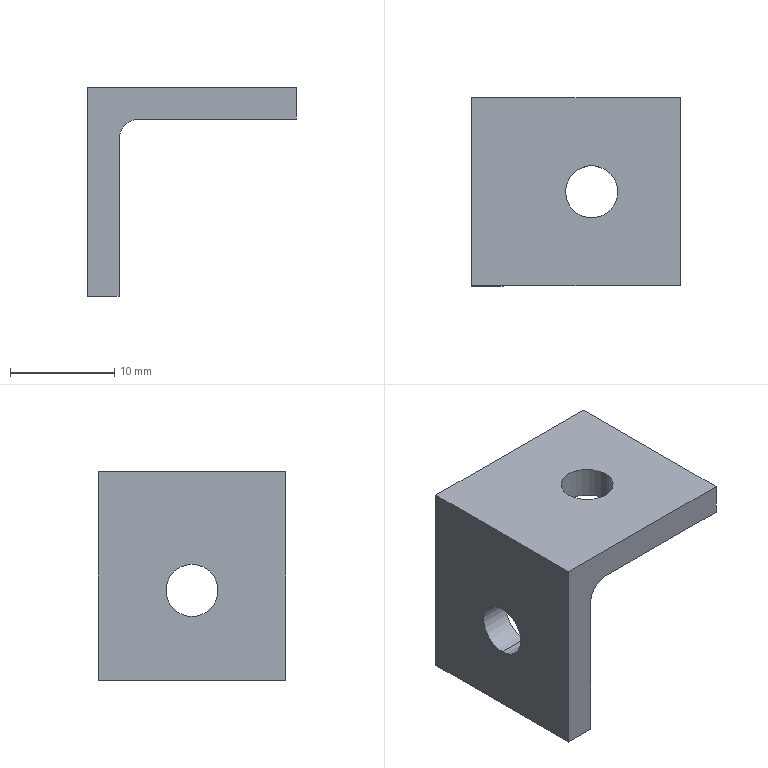Part | STEP file | 20 angle bracket flat | 1 solid | 13 faces | box 20 x 18 x 20 mm | volume 1896 mm3 | plane 8 | cylinder 5 | commonest cylinder face diameters 5 x4 4 x1
STEP:
#1=CARTESIAN_POINT('',(0.,0.,0.));
#2=DIRECTION('',(0.,0.,1.));
#3=DIRECTION('',(1.,0.,0.));
#4=AXIS2_PLACEMENT_3D('',#1,#2,#3);
#5=CARTESIAN_POINT('',(0.,9.,-13.886));
#6=VERTEX_POINT('',#5);
#7=CARTESIAN_POINT('',(3.,9.,-13.886));
#8=VERTEX_POINT('',#7);
#9=CARTESIAN_POINT('',(-7.,9.,-13.886));
#10=DIRECTION('',(1.,0.,0.));
#11=VECTOR('',#10,1.);
#12=LINE('',#9,#11);
#13=CARTESIAN_POINT('',(-7.,9.,-11.386));
#14=DIRECTION('',(1.,0.,0.));
#15=DIRECTION('',(0.,0.,-1.));
#16=AXIS2_PLACEMENT_3D('',#13,#14,#15);
#17=CYLINDRICAL_SURFACE('',#16,2.5);
#18=CARTESIAN_POINT('',(6.283,0.));
#19=DIRECTION('',(0.,1.));
#20=VECTOR('',#19,1.);
#21=LINE('',#18,#20);
#22=(GEOMETRIC_REPRESENTATION_CONTEXT(2)PARAMETRIC_REPRESENTATION_CONTEXT()REPRESENTATION_CONTEXT('',''));
#23=DEFINITIONAL_REPRESENTATION('',(#21),#22);
#24=PCURVE('',#17,#23);
#25=CARTESIAN_POINT('',(-7.,9.,-11.386));
#26=DIRECTION('',(1.,0.,0.));
#27=DIRECTION('',(0.,0.,-1.));
#28=AXIS2_PLACEMENT_3D('',#25,#26,#27);
#29=CYLINDRICAL_SURFACE('',#28,2.5);
#30=CARTESIAN_POINT('',(0.,0.));
#31=DIRECTION('',(0.,1.));
#32=VECTOR('',#31,1.);
#33=LINE('',#30,#32);
#34=(GEOMETRIC_REPRESENTATION_CONTEXT(2)PARAMETRIC_REPRESENTATION_CONTEXT()REPRESENTATION_CONTEXT('',''));
#35=DEFINITIONAL_REPRESENTATION('',(#33),#34);
#36=PCURVE('',#29,#35);
#37=SURFACE_CURVE('',#12,(#24,#36),.PCURVE_S1.);
#38=EDGE_CURVE('',#6,#8,#37,.T.);
#39=ORIENTED_EDGE('',*,*,#38,.T.);
#40=CARTESIAN_POINT('',(3.,9.,-8.886));
#41=VERTEX_POINT('',#40);
#42=CARTESIAN_POINT('',(3.,9.,-11.386));
#43=DIRECTION('',(1.,0.,0.));
#44=DIRECTION('',(0.,0.,-1.));
#45=AXIS2_PLACEMENT_3D('',#42,#43,#44);
#46=CIRCLE('',#45,2.5);
#47=CARTESIAN_POINT('',(0.,10.));
#48=DIRECTION('',(1.,0.));
#49=VECTOR('',#48,1.);
#50=LINE('',#47,#49);
#51=(GEOMETRIC_REPRESENTATION_CONTEXT(2)PARAMETRIC_REPRESENTATION_CONTEXT()REPRESENTATION_CONTEXT('',''));
#52=DEFINITIONAL_REPRESENTATION('',(#50),#51);
#53=PCURVE('',#17,#52);
#54=CARTESIAN_POINT('',(3.,18.,-20.));
#55=DIRECTION('',(1.,0.,0.));
#56=DIRECTION('',(0.,0.,-1.));
#57=AXIS2_PLACEMENT_3D('',#54,#55,#56);
#58=PLANE('',#57);
#59=CARTESIAN_POINT('',(-8.614,-9.));
#60=DIRECTION('',(1.,0.));
#61=AXIS2_PLACEMENT_2D('',#59,#60);
#62=CIRCLE('',#61,2.5);
#63=(GEOMETRIC_REPRESENTATION_CONTEXT(2)PARAMETRIC_REPRESENTATION_CONTEXT()REPRESENTATION_CONTEXT('',''));
#64=DEFINITIONAL_REPRESENTATION('',(#62),#63);
#65=PCURVE('',#58,#64);
#66=SURFACE_CURVE('',#46,(#53,#65),.PCURVE_S1.);
#67=EDGE_CURVE('',#41,#8,#66,.T.);
#68=ORIENTED_EDGE('',*,*,#67,.F.);
#69=CARTESIAN_POINT('',(0.,9.,-8.886));
#70=VERTEX_POINT('',#69);
#71=CARTESIAN_POINT('',(-7.,9.,-8.886));
#72=DIRECTION('',(1.,0.,0.));
#73=VECTOR('',#72,1.);
#74=LINE('',#71,#73);
#75=CARTESIAN_POINT('',(3.142,0.));
#76=DIRECTION('',(0.,1.));
#77=VECTOR('',#76,1.);
#78=LINE('',#75,#77);
#79=(GEOMETRIC_REPRESENTATION_CONTEXT(2)PARAMETRIC_REPRESENTATION_CONTEXT()REPRESENTATION_CONTEXT('',''));
#80=DEFINITIONAL_REPRESENTATION('',(#78),#79);
#81=PCURVE('',#17,#80);
#82=CARTESIAN_POINT('',(3.142,0.));
#83=DIRECTION('',(0.,1.));
#84=VECTOR('',#83,1.);
#85=LINE('',#82,#84);
#86=(GEOMETRIC_REPRESENTATION_CONTEXT(2)PARAMETRIC_REPRESENTATION_CONTEXT()REPRESENTATION_CONTEXT('',''));
#87=DEFINITIONAL_REPRESENTATION('',(#85),#86);
#88=PCURVE('',#29,#87);
#89=SURFACE_CURVE('',#74,(#81,#88),.PCURVE_S1.);
#90=EDGE_CURVE('',#70,#41,#89,.T.);
#91=ORIENTED_EDGE('',*,*,#90,.F.);
#92=CARTESIAN_POINT('',(0.,9.,-11.386));
#93=DIRECTION('',(1.,0.,0.));
#94=DIRECTION('',(0.,0.,-1.));
#95=AXIS2_PLACEMENT_3D('',#92,#93,#94);
#96=CIRCLE('',#95,2.5);
#97=CARTESIAN_POINT('',(0.,7.));
#98=DIRECTION('',(1.,0.));
#99=VECTOR('',#98,1.);
#100=LINE('',#97,#99);
#101=(GEOMETRIC_REPRESENTATION_CONTEXT(2)PARAMETRIC_REPRESENTATION_CONTEXT()REPRESENTATION_CONTEXT('',''));
#102=DEFINITIONAL_REPRESENTATION('',(#100),#101);
#103=PCURVE('',#17,#102);
#104=CARTESIAN_POINT('',(0.,18.,-20.));
#105=DIRECTION('',(1.,0.,0.));
#106=DIRECTION('',(0.,0.,-1.));
#107=AXIS2_PLACEMENT_3D('',#104,#105,#106);
#108=PLANE('',#107);
#109=CARTESIAN_POINT('',(-8.614,-9.));
#110=DIRECTION('',(1.,0.));
#111=AXIS2_PLACEMENT_2D('',#109,#110);
#112=CIRCLE('',#111,2.5);
#113=(GEOMETRIC_REPRESENTATION_CONTEXT(2)PARAMETRIC_REPRESENTATION_CONTEXT()REPRESENTATION_CONTEXT('',''));
#114=DEFINITIONAL_REPRESENTATION('',(#112),#113);
#115=PCURVE('',#108,#114);
#116=SURFACE_CURVE('',#96,(#103,#115),.PCURVE_S1.);
#117=EDGE_CURVE('',#70,#6,#116,.T.);
#118=ORIENTED_EDGE('',*,*,#117,.T.);
#119=EDGE_LOOP('',(#39,#68,#91,#118));
#120=FACE_BOUND('',#119,.F.);
#121=ADVANCED_FACE('',(#120),#17,.F.);
#122=CARTESIAN_POINT('',(9.,9.,0.));
#123=VERTEX_POINT('',#122);
#124=CARTESIAN_POINT('',(9.,9.,-3.));
#125=VERTEX_POINT('',#124);
#126=CARTESIAN_POINT('',(9.,9.,7.));
#127=DIRECTION('',(0.,0.,-1.));
#128=VECTOR('',#127,1.);
#129=LINE('',#126,#128);
#130=CARTESIAN_POINT('',(11.5,9.,7.));
#131=DIRECTION('',(0.,0.,-1.));
#132=DIRECTION('',(-1.,0.,0.));
#133=AXIS2_PLACEMENT_3D('',#130,#131,#132);
#134=CYLINDRICAL_SURFACE('',#133,2.5);
#135=CARTESIAN_POINT('',(6.283,0.));
#136=DIRECTION('',(0.,1.));
#137=VECTOR('',#136,1.);
#138=LINE('',#135,#137);
#139=(GEOMETRIC_REPRESENTATION_CONTEXT(2)PARAMETRIC_REPRESENTATION_CONTEXT()REPRESENTATION_CONTEXT('',''));
#140=DEFINITIONAL_REPRESENTATION('',(#138),#139);
#141=PCURVE('',#134,#140);
#142=CARTESIAN_POINT('',(11.5,9.,7.));
#143=DIRECTION('',(0.,0.,-1.));
#144=DIRECTION('',(-1.,0.,0.));
#145=AXIS2_PLACEMENT_3D('',#142,#143,#144);
#146=CYLINDRICAL_SURFACE('',#145,2.5);
#147=CARTESIAN_POINT('',(0.,0.));
#148=DIRECTION('',(0.,1.));
#149=VECTOR('',#148,1.);
#150=LINE('',#147,#149);
#151=(GEOMETRIC_REPRESENTATION_CONTEXT(2)PARAMETRIC_REPRESENTATION_CONTEXT()REPRESENTATION_CONTEXT('',''));
#152=DEFINITIONAL_REPRESENTATION('',(#150),#151);
#153=PCURVE('',#146,#152);
#154=SURFACE_CURVE('',#129,(#141,#153),.PCURVE_S1.);
#155=EDGE_CURVE('',#123,#125,#154,.T.);
#156=ORIENTED_EDGE('',*,*,#155,.T.);
#157=CARTESIAN_POINT('',(14.,9.,-3.));
#158=VERTEX_POINT('',#157);
#159=CARTESIAN_POINT('',(11.5,9.,-3.));
#160=DIRECTION('',(0.,0.,-1.));
#161=DIRECTION('',(-1.,0.,0.));
#162=AXIS2_PLACEMENT_3D('',#159,#160,#161);
#163=CIRCLE('',#162,2.5);
#164=CARTESIAN_POINT('',(0.,10.));
#165=DIRECTION('',(1.,0.));
#166=VECTOR('',#165,1.);
#167=LINE('',#164,#166);
#168=(GEOMETRIC_REPRESENTATION_CONTEXT(2)PARAMETRIC_REPRESENTATION_CONTEXT()REPRESENTATION_CONTEXT('',''));
#169=DEFINITIONAL_REPRESENTATION('',(#167),#168);
#170=PCURVE('',#134,#169);
#171=CARTESIAN_POINT('',(0.,18.,-3.));
#172=DIRECTION('',(0.,0.,-1.));
#173=DIRECTION('',(-1.,0.,0.));
#174=AXIS2_PLACEMENT_3D('',#171,#172,#173);
#175=PLANE('',#174);
#176=CARTESIAN_POINT('',(-11.5,-9.));
#177=DIRECTION('',(1.,0.));
#178=AXIS2_PLACEMENT_2D('',#176,#177);
#179=CIRCLE('',#178,2.5);
#180=(GEOMETRIC_REPRESENTATION_CONTEXT(2)PARAMETRIC_REPRESENTATION_CONTEXT()REPRESENTATION_CONTEXT('',''));
#181=DEFINITIONAL_REPRESENTATION('',(#179),#180);
#182=PCURVE('',#175,#181);
#183=SURFACE_CURVE('',#163,(#170,#182),.PCURVE_S1.);
#184=EDGE_CURVE('',#158,#125,#183,.T.);
#185=ORIENTED_EDGE('',*,*,#184,.F.);
#186=CARTESIAN_POINT('',(14.,9.,0.));
#187=VERTEX_POINT('',#186);
#188=CARTESIAN_POINT('',(14.,9.,7.));
#189=DIRECTION('',(0.,0.,-1.));
#190=VECTOR('',#189,1.);
#191=LINE('',#188,#190);
#192=CARTESIAN_POINT('',(3.142,0.));
#193=DIRECTION('',(0.,1.));
#194=VECTOR('',#193,1.);
#195=LINE('',#192,#194);
#196=(GEOMETRIC_REPRESENTATION_CONTEXT(2)PARAMETRIC_REPRESENTATION_CONTEXT()REPRESENTATION_CONTEXT('',''));
#197=DEFINITIONAL_REPRESENTATION('',(#195),#196);
#198=PCURVE('',#134,#197);
#199=CARTESIAN_POINT('',(3.142,0.));
#200=DIRECTION('',(0.,1.));
#201=VECTOR('',#200,1.);
#202=LINE('',#199,#201);
#203=(GEOMETRIC_REPRESENTATION_CONTEXT(2)PARAMETRIC_REPRESENTATION_CONTEXT()REPRESENTATION_CONTEXT('',''));
#204=DEFINITIONAL_REPRESENTATION('',(#202),#203);
#205=PCURVE('',#146,#204);
#206=SURFACE_CURVE('',#191,(#198,#205),.PCURVE_S1.);
#207=EDGE_CURVE('',#187,#158,#206,.T.);
#208=ORIENTED_EDGE('',*,*,#207,.F.);
#209=CARTESIAN_POINT('',(11.5,9.,0.));
#210=DIRECTION('',(0.,0.,-1.));
#211=DIRECTION('',(-1.,0.,0.));
#212=AXIS2_PLACEMENT_3D('',#209,#210,#211);
#213=CIRCLE('',#212,2.5);
#214=CARTESIAN_POINT('',(0.,7.));
#215=DIRECTION('',(1.,0.));
#216=VECTOR('',#215,1.);
#217=LINE('',#214,#216);
#218=(GEOMETRIC_REPRESENTATION_CONTEXT(2)PARAMETRIC_REPRESENTATION_CONTEXT()REPRESENTATION_CONTEXT('',''));
#219=DEFINITIONAL_REPRESENTATION('',(#217),#218);
#220=PCURVE('',#134,#219);
#221=CARTESIAN_POINT('',(0.,18.,0.));
#222=DIRECTION('',(0.,0.,-1.));
#223=DIRECTION('',(-1.,0.,0.));
#224=AXIS2_PLACEMENT_3D('',#221,#222,#223);
#225=PLANE('',#224);
#226=CARTESIAN_POINT('',(-11.5,-9.));
#227=DIRECTION('',(1.,0.));
#228=AXIS2_PLACEMENT_2D('',#226,#227);
#229=CIRCLE('',#228,2.5);
#230=(GEOMETRIC_REPRESENTATION_CONTEXT(2)PARAMETRIC_REPRESENTATION_CONTEXT()REPRESENTATION_CONTEXT('',''));
#231=DEFINITIONAL_REPRESENTATION('',(#229),#230);
#232=PCURVE('',#225,#231);
#233=SURFACE_CURVE('',#213,(#220,#232),.PCURVE_S1.);
#234=EDGE_CURVE('',#187,#123,#233,.T.);
#235=ORIENTED_EDGE('',*,*,#234,.T.);
#236=EDGE_LOOP('',(#156,#185,#208,#235));
#237=FACE_BOUND('',#236,.F.);
#238=ADVANCED_FACE('',(#237),#134,.F.);
#239=CARTESIAN_POINT('',(11.5,9.,0.));
#240=DIRECTION('',(0.,0.,-1.));
#241=DIRECTION('',(-1.,0.,0.));
#242=AXIS2_PLACEMENT_3D('',#239,#240,#241);
#243=CIRCLE('',#242,2.5);
#244=CARTESIAN_POINT('',(-11.5,-9.));
#245=DIRECTION('',(1.,0.));
#246=AXIS2_PLACEMENT_2D('',#244,#245);
#247=CIRCLE('',#246,2.5);
#248=(GEOMETRIC_REPRESENTATION_CONTEXT(2)PARAMETRIC_REPRESENTATION_CONTEXT()REPRESENTATION_CONTEXT('',''));
#249=DEFINITIONAL_REPRESENTATION('',(#247),#248);
#250=PCURVE('',#225,#249);
#251=CARTESIAN_POINT('',(0.,7.));
#252=DIRECTION('',(1.,0.));
#253=VECTOR('',#252,1.);
#254=LINE('',#251,#253);
#255=(GEOMETRIC_REPRESENTATION_CONTEXT(2)PARAMETRIC_REPRESENTATION_CONTEXT()REPRESENTATION_CONTEXT('',''));
#256=DEFINITIONAL_REPRESENTATION('',(#254),#255);
#257=PCURVE('',#146,#256);
#258=SURFACE_CURVE('',#243,(#250,#257),.PCURVE_S1.);
#259=EDGE_CURVE('',#123,#187,#258,.T.);
#260=ORIENTED_EDGE('',*,*,#259,.T.);
#261=ORIENTED_EDGE('',*,*,#234,.T.);
#262=EDGE_LOOP('',(#260,#261));
#263=FACE_BOUND('',#262,.T.);
#264=CARTESIAN_POINT('',(0.,0.,0.));
#265=VERTEX_POINT('',#264);
#266=CARTESIAN_POINT('',(20.,0.,0.));
#267=VERTEX_POINT('',#266);
#268=CARTESIAN_POINT('',(0.,0.,0.));
#269=DIRECTION('',(1.,0.,0.));
#270=VECTOR('',#269,1.);
#271=LINE('',#268,#270);
#272=CARTESIAN_POINT('',(0.,-18.));
#273=DIRECTION('',(-1.,0.));
#274=VECTOR('',#273,1.);
#275=LINE('',#272,#274);
#276=(GEOMETRIC_REPRESENTATION_CONTEXT(2)PARAMETRIC_REPRESENTATION_CONTEXT()REPRESENTATION_CONTEXT('',''));
#277=DEFINITIONAL_REPRESENTATION('',(#275),#276);
#278=PCURVE('',#225,#277);
#279=CARTESIAN_POINT('',(0.,0.,0.));
#280=DIRECTION('',(0.,-1.,0.));
#281=DIRECTION('',(-1.,0.,0.));
#282=AXIS2_PLACEMENT_3D('',#279,#280,#281);
#283=PLANE('',#282);
#284=CARTESIAN_POINT('',(0.,0.));
#285=DIRECTION('',(-1.,0.));
#286=VECTOR('',#285,1.);
#287=LINE('',#284,#286);
#288=(GEOMETRIC_REPRESENTATION_CONTEXT(2)PARAMETRIC_REPRESENTATION_CONTEXT()REPRESENTATION_CONTEXT('',''));
#289=DEFINITIONAL_REPRESENTATION('',(#287),#288);
#290=PCURVE('',#283,#289);
#291=SURFACE_CURVE('',#271,(#278,#290),.PCURVE_S1.);
#292=EDGE_CURVE('',#265,#267,#291,.T.);
#293=ORIENTED_EDGE('',*,*,#292,.T.);
#294=CARTESIAN_POINT('',(20.,18.,0.));
#295=VERTEX_POINT('',#294);
#296=CARTESIAN_POINT('',(20.,18.,0.));
#297=DIRECTION('',(0.,-1.,0.));
#298=VECTOR('',#297,1.);
#299=LINE('',#296,#298);
#300=CARTESIAN_POINT('',(-20.,0.));
#301=DIRECTION('',(0.,-1.));
#302=VECTOR('',#301,1.);
#303=LINE('',#300,#302);
#304=(GEOMETRIC_REPRESENTATION_CONTEXT(2)PARAMETRIC_REPRESENTATION_CONTEXT()REPRESENTATION_CONTEXT('',''));
#305=DEFINITIONAL_REPRESENTATION('',(#303),#304);
#306=PCURVE('',#225,#305);
#307=CARTESIAN_POINT('',(20.,18.,-3.));
#308=DIRECTION('',(1.,0.,0.));
#309=DIRECTION('',(0.,0.,-1.));
#310=AXIS2_PLACEMENT_3D('',#307,#308,#309);
#311=PLANE('',#310);
#312=CARTESIAN_POINT('',(-3.,0.));
#313=DIRECTION('',(0.,-1.));
#314=VECTOR('',#313,1.);
#315=LINE('',#312,#314);
#316=(GEOMETRIC_REPRESENTATION_CONTEXT(2)PARAMETRIC_REPRESENTATION_CONTEXT()REPRESENTATION_CONTEXT('',''));
#317=DEFINITIONAL_REPRESENTATION('',(#315),#316);
#318=PCURVE('',#311,#317);
#319=SURFACE_CURVE('',#299,(#306,#318),.PCURVE_S1.);
#320=EDGE_CURVE('',#295,#267,#319,.T.);
#321=ORIENTED_EDGE('',*,*,#320,.F.);
#322=CARTESIAN_POINT('',(0.,18.,0.));
#323=VERTEX_POINT('',#322);
#324=CARTESIAN_POINT('',(0.,18.,0.));
#325=DIRECTION('',(1.,0.,0.));
#326=VECTOR('',#325,1.);
#327=LINE('',#324,#326);
#328=CARTESIAN_POINT('',(0.,0.));
#329=DIRECTION('',(-1.,0.));
#330=VECTOR('',#329,1.);
#331=LINE('',#328,#330);
#332=(GEOMETRIC_REPRESENTATION_CONTEXT(2)PARAMETRIC_REPRESENTATION_CONTEXT()REPRESENTATION_CONTEXT('',''));
#333=DEFINITIONAL_REPRESENTATION('',(#331),#332);
#334=PCURVE('',#225,#333);
#335=CARTESIAN_POINT('',(0.,18.,0.));
#336=DIRECTION('',(0.,-1.,0.));
#337=DIRECTION('',(-1.,0.,0.));
#338=AXIS2_PLACEMENT_3D('',#335,#336,#337);
#339=PLANE('',#338);
#340=CARTESIAN_POINT('',(0.,0.));
#341=DIRECTION('',(-1.,0.));
#342=VECTOR('',#341,1.);
#343=LINE('',#340,#342);
#344=(GEOMETRIC_REPRESENTATION_CONTEXT(2)PARAMETRIC_REPRESENTATION_CONTEXT()REPRESENTATION_CONTEXT('',''));
#345=DEFINITIONAL_REPRESENTATION('',(#343),#344);
#346=PCURVE('',#339,#345);
#347=SURFACE_CURVE('',#327,(#334,#346),.PCURVE_S1.);
#348=EDGE_CURVE('',#323,#295,#347,.T.);
#349=ORIENTED_EDGE('',*,*,#348,.F.);
#350=CARTESIAN_POINT('',(0.,18.,0.));
#351=DIRECTION('',(0.,-1.,0.));
#352=VECTOR('',#351,1.);
#353=LINE('',#350,#352);
#354=CARTESIAN_POINT('',(0.,0.));
#355=DIRECTION('',(0.,-1.));
#356=VECTOR('',#355,1.);
#357=LINE('',#354,#356);
#358=(GEOMETRIC_REPRESENTATION_CONTEXT(2)PARAMETRIC_REPRESENTATION_CONTEXT()REPRESENTATION_CONTEXT('',''));
#359=DEFINITIONAL_REPRESENTATION('',(#357),#358);
#360=PCURVE('',#225,#359);
#361=CARTESIAN_POINT('',(-20.,0.));
#362=DIRECTION('',(0.,-1.));
#363=VECTOR('',#362,1.);
#364=LINE('',#361,#363);
#365=(GEOMETRIC_REPRESENTATION_CONTEXT(2)PARAMETRIC_REPRESENTATION_CONTEXT()REPRESENTATION_CONTEXT('',''));
#366=DEFINITIONAL_REPRESENTATION('',(#364),#365);
#367=PCURVE('',#108,#366);
#368=SURFACE_CURVE('',#353,(#360,#367),.PCURVE_S1.);
#369=EDGE_CURVE('',#323,#265,#368,.T.);
#370=ORIENTED_EDGE('',*,*,#369,.T.);
#371=EDGE_LOOP('',(#293,#321,#349,#370));
#372=FACE_BOUND('',#371,.T.);
#373=ADVANCED_FACE('',(#263,#372),#225,.F.);
#374=CARTESIAN_POINT('',(20.,0.,-3.));
#375=VERTEX_POINT('',#374);
#376=CARTESIAN_POINT('',(20.,0.,-3.));
#377=DIRECTION('',(0.,0.,1.));
#378=VECTOR('',#377,1.);
#379=LINE('',#376,#378);
#380=CARTESIAN_POINT('',(0.,-18.));
#381=DIRECTION('',(-1.,0.));
#382=VECTOR('',#381,1.);
#383=LINE('',#380,#382);
#384=(GEOMETRIC_REPRESENTATION_CONTEXT(2)PARAMETRIC_REPRESENTATION_CONTEXT()REPRESENTATION_CONTEXT('',''));
#385=DEFINITIONAL_REPRESENTATION('',(#383),#384);
#386=PCURVE('',#311,#385);
#387=CARTESIAN_POINT('',(-20.,3.));
#388=DIRECTION('',(0.,-1.));
#389=VECTOR('',#388,1.);
#390=LINE('',#387,#389);
#391=(GEOMETRIC_REPRESENTATION_CONTEXT(2)PARAMETRIC_REPRESENTATION_CONTEXT()REPRESENTATION_CONTEXT('',''));
#392=DEFINITIONAL_REPRESENTATION('',(#390),#391);
#393=PCURVE('',#283,#392);
#394=SURFACE_CURVE('',#379,(#386,#393),.PCURVE_S1.);
#395=EDGE_CURVE('',#375,#267,#394,.T.);
#396=ORIENTED_EDGE('',*,*,#395,.F.);
#397=CARTESIAN_POINT('',(20.,18.,-3.));
#398=VERTEX_POINT('',#397);
#399=CARTESIAN_POINT('',(20.,18.,-3.));
#400=DIRECTION('',(0.,-1.,0.));
#401=VECTOR('',#400,1.);
#402=LINE('',#399,#401);
#403=CARTESIAN_POINT('',(0.,0.));
#404=DIRECTION('',(0.,-1.));
#405=VECTOR('',#404,1.);
#406=LINE('',#403,#405);
#407=(GEOMETRIC_REPRESENTATION_CONTEXT(2)PARAMETRIC_REPRESENTATION_CONTEXT()REPRESENTATION_CONTEXT('',''));
#408=DEFINITIONAL_REPRESENTATION('',(#406),#407);
#409=PCURVE('',#311,#408);
#410=CARTESIAN_POINT('',(-20.,0.));
#411=DIRECTION('',(0.,-1.));
#412=VECTOR('',#411,1.);
#413=LINE('',#410,#412);
#414=(GEOMETRIC_REPRESENTATION_CONTEXT(2)PARAMETRIC_REPRESENTATION_CONTEXT()REPRESENTATION_CONTEXT('',''));
#415=DEFINITIONAL_REPRESENTATION('',(#413),#414);
#416=PCURVE('',#175,#415);
#417=SURFACE_CURVE('',#402,(#409,#416),.PCURVE_S1.);
#418=EDGE_CURVE('',#398,#375,#417,.T.);
#419=ORIENTED_EDGE('',*,*,#418,.F.);
#420=CARTESIAN_POINT('',(20.,18.,-3.));
#421=DIRECTION('',(0.,0.,1.));
#422=VECTOR('',#421,1.);
#423=LINE('',#420,#422);
#424=CARTESIAN_POINT('',(0.,0.));
#425=DIRECTION('',(-1.,0.));
#426=VECTOR('',#425,1.);
#427=LINE('',#424,#426);
#428=(GEOMETRIC_REPRESENTATION_CONTEXT(2)PARAMETRIC_REPRESENTATION_CONTEXT()REPRESENTATION_CONTEXT('',''));
#429=DEFINITIONAL_REPRESENTATION('',(#427),#428);
#430=PCURVE('',#311,#429);
#431=CARTESIAN_POINT('',(-20.,3.));
#432=DIRECTION('',(0.,-1.));
#433=VECTOR('',#432,1.);
#434=LINE('',#431,#433);
#435=(GEOMETRIC_REPRESENTATION_CONTEXT(2)PARAMETRIC_REPRESENTATION_CONTEXT()REPRESENTATION_CONTEXT('',''));
#436=DEFINITIONAL_REPRESENTATION('',(#434),#435);
#437=PCURVE('',#339,#436);
#438=SURFACE_CURVE('',#423,(#430,#437),.PCURVE_S1.);
#439=EDGE_CURVE('',#398,#295,#438,.T.);
#440=ORIENTED_EDGE('',*,*,#439,.T.);
#441=ORIENTED_EDGE('',*,*,#320,.T.);
#442=EDGE_LOOP('',(#396,#419,#440,#441));
#443=FACE_BOUND('',#442,.T.);
#444=ADVANCED_FACE('',(#443),#311,.T.);
#445=CARTESIAN_POINT('',(11.5,9.,-3.));
#446=DIRECTION('',(0.,0.,-1.));
#447=DIRECTION('',(-1.,0.,0.));
#448=AXIS2_PLACEMENT_3D('',#445,#446,#447);
#449=CIRCLE('',#448,2.5);
#450=CARTESIAN_POINT('',(-11.5,-9.));
#451=DIRECTION('',(1.,0.));
#452=AXIS2_PLACEMENT_2D('',#450,#451);
#453=CIRCLE('',#452,2.5);
#454=(GEOMETRIC_REPRESENTATION_CONTEXT(2)PARAMETRIC_REPRESENTATION_CONTEXT()REPRESENTATION_CONTEXT('',''));
#455=DEFINITIONAL_REPRESENTATION('',(#453),#454);
#456=PCURVE('',#175,#455);
#457=CARTESIAN_POINT('',(0.,10.));
#458=DIRECTION('',(1.,0.));
#459=VECTOR('',#458,1.);
#460=LINE('',#457,#459);
#461=(GEOMETRIC_REPRESENTATION_CONTEXT(2)PARAMETRIC_REPRESENTATION_CONTEXT()REPRESENTATION_CONTEXT('',''));
#462=DEFINITIONAL_REPRESENTATION('',(#460),#461);
#463=PCURVE('',#146,#462);
#464=SURFACE_CURVE('',#449,(#456,#463),.PCURVE_S1.);
#465=EDGE_CURVE('',#125,#158,#464,.T.);
#466=ORIENTED_EDGE('',*,*,#465,.F.);
#467=ORIENTED_EDGE('',*,*,#184,.F.);
#468=EDGE_LOOP('',(#466,#467));
#469=FACE_BOUND('',#468,.T.);
#470=CARTESIAN_POINT('',(5.,0.,-3.));
#471=VERTEX_POINT('',#470);
#472=CARTESIAN_POINT('',(0.,0.,-3.));
#473=DIRECTION('',(1.,0.,0.));
#474=VECTOR('',#473,1.);
#475=LINE('',#472,#474);
#476=CARTESIAN_POINT('',(0.,-18.));
#477=DIRECTION('',(-1.,0.));
#478=VECTOR('',#477,1.);
#479=LINE('',#476,#478);
#480=(GEOMETRIC_REPRESENTATION_CONTEXT(2)PARAMETRIC_REPRESENTATION_CONTEXT()REPRESENTATION_CONTEXT('',''));
#481=DEFINITIONAL_REPRESENTATION('',(#479),#480);
#482=PCURVE('',#175,#481);
#483=CARTESIAN_POINT('',(0.,3.));
#484=DIRECTION('',(-1.,0.));
#485=VECTOR('',#484,1.);
#486=LINE('',#483,#485);
#487=(GEOMETRIC_REPRESENTATION_CONTEXT(2)PARAMETRIC_REPRESENTATION_CONTEXT()REPRESENTATION_CONTEXT('',''));
#488=DEFINITIONAL_REPRESENTATION('',(#486),#487);
#489=PCURVE('',#283,#488);
#490=SURFACE_CURVE('',#475,(#482,#489),.PCURVE_S1.);
#491=EDGE_CURVE('',#471,#375,#490,.T.);
#492=ORIENTED_EDGE('',*,*,#491,.F.);
#493=CARTESIAN_POINT('',(5.,18.,-3.));
#494=VERTEX_POINT('',#493);
#495=CARTESIAN_POINT('',(5.,18.,-3.));
#496=DIRECTION('',(0.,1.,0.));
#497=VECTOR('',#496,1.);
#498=LINE('',#495,#497);
#499=CARTESIAN_POINT('',(-5.,0.));
#500=DIRECTION('',(0.,1.));
#501=VECTOR('',#500,1.);
#502=LINE('',#499,#501);
#503=(GEOMETRIC_REPRESENTATION_CONTEXT(2)PARAMETRIC_REPRESENTATION_CONTEXT()REPRESENTATION_CONTEXT('',''));
#504=DEFINITIONAL_REPRESENTATION('',(#502),#503);
#505=PCURVE('',#175,#504);
#506=CARTESIAN_POINT('',(5.,18.,-5.));
#507=DIRECTION('',(0.,1.,0.));
#508=DIRECTION('',(0.,0.,1.));
#509=AXIS2_PLACEMENT_3D('',#506,#507,#508);
#510=CYLINDRICAL_SURFACE('',#509,2.);
#511=CARTESIAN_POINT('',(6.283,0.));
#512=DIRECTION('',(0.,1.));
#513=VECTOR('',#512,1.);
#514=LINE('',#511,#513);
#515=(GEOMETRIC_REPRESENTATION_CONTEXT(2)PARAMETRIC_REPRESENTATION_CONTEXT()REPRESENTATION_CONTEXT('',''));
#516=DEFINITIONAL_REPRESENTATION('',(#514),#515);
#517=PCURVE('',#510,#516);
#518=SURFACE_CURVE('',#498,(#505,#517),.PCURVE_S1.);
#519=EDGE_CURVE('',#471,#494,#518,.T.);
#520=ORIENTED_EDGE('',*,*,#519,.T.);
#521=CARTESIAN_POINT('',(0.,18.,-3.));
#522=DIRECTION('',(1.,0.,0.));
#523=VECTOR('',#522,1.);
#524=LINE('',#521,#523);
#525=CARTESIAN_POINT('',(0.,0.));
#526=DIRECTION('',(-1.,0.));
#527=VECTOR('',#526,1.);
#528=LINE('',#525,#527);
#529=(GEOMETRIC_REPRESENTATION_CONTEXT(2)PARAMETRIC_REPRESENTATION_CONTEXT()REPRESENTATION_CONTEXT('',''));
#530=DEFINITIONAL_REPRESENTATION('',(#528),#529);
#531=PCURVE('',#175,#530);
#532=CARTESIAN_POINT('',(0.,3.));
#533=DIRECTION('',(-1.,0.));
#534=VECTOR('',#533,1.);
#535=LINE('',#532,#534);
#536=(GEOMETRIC_REPRESENTATION_CONTEXT(2)PARAMETRIC_REPRESENTATION_CONTEXT()REPRESENTATION_CONTEXT('',''));
#537=DEFINITIONAL_REPRESENTATION('',(#535),#536);
#538=PCURVE('',#339,#537);
#539=SURFACE_CURVE('',#524,(#531,#538),.PCURVE_S1.);
#540=EDGE_CURVE('',#494,#398,#539,.T.);
#541=ORIENTED_EDGE('',*,*,#540,.T.);
#542=ORIENTED_EDGE('',*,*,#418,.T.);
#543=EDGE_LOOP('',(#492,#520,#541,#542));
#544=FACE_BOUND('',#543,.T.);
#545=ADVANCED_FACE('',(#469,#544),#175,.T.);
#546=CARTESIAN_POINT('',(3.,9.,-11.386));
#547=DIRECTION('',(1.,0.,0.));
#548=DIRECTION('',(0.,0.,-1.));
#549=AXIS2_PLACEMENT_3D('',#546,#547,#548);
#550=CIRCLE('',#549,2.5);
#551=CARTESIAN_POINT('',(-8.614,-9.));
#552=DIRECTION('',(1.,0.));
#553=AXIS2_PLACEMENT_2D('',#551,#552);
#554=CIRCLE('',#553,2.5);
#555=(GEOMETRIC_REPRESENTATION_CONTEXT(2)PARAMETRIC_REPRESENTATION_CONTEXT()REPRESENTATION_CONTEXT('',''));
#556=DEFINITIONAL_REPRESENTATION('',(#554),#555);
#557=PCURVE('',#58,#556);
#558=CARTESIAN_POINT('',(0.,10.));
#559=DIRECTION('',(1.,0.));
#560=VECTOR('',#559,1.);
#561=LINE('',#558,#560);
#562=(GEOMETRIC_REPRESENTATION_CONTEXT(2)PARAMETRIC_REPRESENTATION_CONTEXT()REPRESENTATION_CONTEXT('',''));
#563=DEFINITIONAL_REPRESENTATION('',(#561),#562);
#564=PCURVE('',#29,#563);
#565=SURFACE_CURVE('',#550,(#557,#564),.PCURVE_S1.);
#566=EDGE_CURVE('',#8,#41,#565,.T.);
#567=ORIENTED_EDGE('',*,*,#566,.F.);
#568=ORIENTED_EDGE('',*,*,#67,.F.);
#569=EDGE_LOOP('',(#567,#568));
#570=FACE_BOUND('',#569,.T.);
#571=CARTESIAN_POINT('',(3.,18.,-20.));
#572=VERTEX_POINT('',#571);
#573=CARTESIAN_POINT('',(3.,18.,-5.));
#574=VERTEX_POINT('',#573);
#575=CARTESIAN_POINT('',(3.,18.,-20.));
#576=DIRECTION('',(0.,0.,1.));
#577=VECTOR('',#576,1.);
#578=LINE('',#575,#577);
#579=CARTESIAN_POINT('',(0.,0.));
#580=DIRECTION('',(-1.,0.));
#581=VECTOR('',#580,1.);
#582=LINE('',#579,#581);
#583=(GEOMETRIC_REPRESENTATION_CONTEXT(2)PARAMETRIC_REPRESENTATION_CONTEXT()REPRESENTATION_CONTEXT('',''));
#584=DEFINITIONAL_REPRESENTATION('',(#582),#583);
#585=PCURVE('',#58,#584);
#586=CARTESIAN_POINT('',(-3.,20.));
#587=DIRECTION('',(0.,-1.));
#588=VECTOR('',#587,1.);
#589=LINE('',#586,#588);
#590=(GEOMETRIC_REPRESENTATION_CONTEXT(2)PARAMETRIC_REPRESENTATION_CONTEXT()REPRESENTATION_CONTEXT('',''));
#591=DEFINITIONAL_REPRESENTATION('',(#589),#590);
#592=PCURVE('',#339,#591);
#593=SURFACE_CURVE('',#578,(#585,#592),.PCURVE_S1.);
#594=EDGE_CURVE('',#572,#574,#593,.T.);
#595=ORIENTED_EDGE('',*,*,#594,.T.);
#596=CARTESIAN_POINT('',(3.,0.,-5.));
#597=VERTEX_POINT('',#596);
#598=CARTESIAN_POINT('',(3.,0.,-5.));
#599=DIRECTION('',(0.,-1.,0.));
#600=VECTOR('',#599,1.);
#601=LINE('',#598,#600);
#602=CARTESIAN_POINT('',(-15.,-18.));
#603=DIRECTION('',(0.,-1.));
#604=VECTOR('',#603,1.);
#605=LINE('',#602,#604);
#606=(GEOMETRIC_REPRESENTATION_CONTEXT(2)PARAMETRIC_REPRESENTATION_CONTEXT()REPRESENTATION_CONTEXT('',''));
#607=DEFINITIONAL_REPRESENTATION('',(#605),#606);
#608=PCURVE('',#58,#607);
#609=CARTESIAN_POINT('',(4.712,-18.));
#610=DIRECTION('',(0.,-1.));
#611=VECTOR('',#610,1.);
#612=LINE('',#609,#611);
#613=(GEOMETRIC_REPRESENTATION_CONTEXT(2)PARAMETRIC_REPRESENTATION_CONTEXT()REPRESENTATION_CONTEXT('',''));
#614=DEFINITIONAL_REPRESENTATION('',(#612),#613);
#615=PCURVE('',#510,#614);
#616=SURFACE_CURVE('',#601,(#608,#615),.PCURVE_S1.);
#617=EDGE_CURVE('',#574,#597,#616,.T.);
#618=ORIENTED_EDGE('',*,*,#617,.T.);
#619=CARTESIAN_POINT('',(3.,0.,-20.));
#620=VERTEX_POINT('',#619);
#621=CARTESIAN_POINT('',(3.,0.,-20.));
#622=DIRECTION('',(0.,0.,1.));
#623=VECTOR('',#622,1.);
#624=LINE('',#621,#623);
#625=CARTESIAN_POINT('',(0.,-18.));
#626=DIRECTION('',(-1.,0.));
#627=VECTOR('',#626,1.);
#628=LINE('',#625,#627);
#629=(GEOMETRIC_REPRESENTATION_CONTEXT(2)PARAMETRIC_REPRESENTATION_CONTEXT()REPRESENTATION_CONTEXT('',''));
#630=DEFINITIONAL_REPRESENTATION('',(#628),#629);
#631=PCURVE('',#58,#630);
#632=CARTESIAN_POINT('',(-3.,20.));
#633=DIRECTION('',(0.,-1.));
#634=VECTOR('',#633,1.);
#635=LINE('',#632,#634);
#636=(GEOMETRIC_REPRESENTATION_CONTEXT(2)PARAMETRIC_REPRESENTATION_CONTEXT()REPRESENTATION_CONTEXT('',''));
#637=DEFINITIONAL_REPRESENTATION('',(#635),#636);
#638=PCURVE('',#283,#637);
#639=SURFACE_CURVE('',#624,(#631,#638),.PCURVE_S1.);
#640=EDGE_CURVE('',#620,#597,#639,.T.);
#641=ORIENTED_EDGE('',*,*,#640,.F.);
#642=CARTESIAN_POINT('',(3.,18.,-20.));
#643=DIRECTION('',(0.,-1.,0.));
#644=VECTOR('',#643,1.);
#645=LINE('',#642,#644);
#646=CARTESIAN_POINT('',(0.,0.));
#647=DIRECTION('',(0.,-1.));
#648=VECTOR('',#647,1.);
#649=LINE('',#646,#648);
#650=(GEOMETRIC_REPRESENTATION_CONTEXT(2)PARAMETRIC_REPRESENTATION_CONTEXT()REPRESENTATION_CONTEXT('',''));
#651=DEFINITIONAL_REPRESENTATION('',(#649),#650);
#652=PCURVE('',#58,#651);
#653=CARTESIAN_POINT('',(0.,18.,-20.));
#654=DIRECTION('',(0.,0.,-1.));
#655=DIRECTION('',(-1.,0.,0.));
#656=AXIS2_PLACEMENT_3D('',#653,#654,#655);
#657=PLANE('',#656);
#658=CARTESIAN_POINT('',(-3.,0.));
#659=DIRECTION('',(0.,-1.));
#660=VECTOR('',#659,1.);
#661=LINE('',#658,#660);
#662=(GEOMETRIC_REPRESENTATION_CONTEXT(2)PARAMETRIC_REPRESENTATION_CONTEXT()REPRESENTATION_CONTEXT('',''));
#663=DEFINITIONAL_REPRESENTATION('',(#661),#662);
#664=PCURVE('',#657,#663);
#665=SURFACE_CURVE('',#645,(#652,#664),.PCURVE_S1.);
#666=EDGE_CURVE('',#572,#620,#665,.T.);
#667=ORIENTED_EDGE('',*,*,#666,.F.);
#668=EDGE_LOOP('',(#595,#618,#641,#667));
#669=FACE_BOUND('',#668,.T.);
#670=ADVANCED_FACE('',(#570,#669),#58,.T.);
#671=CARTESIAN_POINT('',(0.,0.,-20.));
#672=VERTEX_POINT('',#671);
#673=CARTESIAN_POINT('',(0.,0.,-20.));
#674=DIRECTION('',(1.,0.,0.));
#675=VECTOR('',#674,1.);
#676=LINE('',#673,#675);
#677=CARTESIAN_POINT('',(0.,-18.));
#678=DIRECTION('',(-1.,0.));
#679=VECTOR('',#678,1.);
#680=LINE('',#677,#679);
#681=(GEOMETRIC_REPRESENTATION_CONTEXT(2)PARAMETRIC_REPRESENTATION_CONTEXT()REPRESENTATION_CONTEXT('',''));
#682=DEFINITIONAL_REPRESENTATION('',(#680),#681);
#683=PCURVE('',#657,#682);
#684=CARTESIAN_POINT('',(0.,20.));
#685=DIRECTION('',(-1.,0.));
#686=VECTOR('',#685,1.);
#687=LINE('',#684,#686);
#688=(GEOMETRIC_REPRESENTATION_CONTEXT(2)PARAMETRIC_REPRESENTATION_CONTEXT()REPRESENTATION_CONTEXT('',''));
#689=DEFINITIONAL_REPRESENTATION('',(#687),#688);
#690=PCURVE('',#283,#689);
#691=SURFACE_CURVE('',#676,(#683,#690),.PCURVE_S1.);
#692=EDGE_CURVE('',#672,#620,#691,.T.);
#693=ORIENTED_EDGE('',*,*,#692,.F.);
#694=CARTESIAN_POINT('',(0.,18.,-20.));
#695=VERTEX_POINT('',#694);
#696=CARTESIAN_POINT('',(0.,18.,-20.));
#697=DIRECTION('',(0.,-1.,0.));
#698=VECTOR('',#697,1.);
#699=LINE('',#696,#698);
#700=CARTESIAN_POINT('',(0.,0.));
#701=DIRECTION('',(0.,-1.));
#702=VECTOR('',#701,1.);
#703=LINE('',#700,#702);
#704=(GEOMETRIC_REPRESENTATION_CONTEXT(2)PARAMETRIC_REPRESENTATION_CONTEXT()REPRESENTATION_CONTEXT('',''));
#705=DEFINITIONAL_REPRESENTATION('',(#703),#704);
#706=PCURVE('',#657,#705);
#707=CARTESIAN_POINT('',(0.,0.));
#708=DIRECTION('',(0.,-1.));
#709=VECTOR('',#708,1.);
#710=LINE('',#707,#709);
#711=(GEOMETRIC_REPRESENTATION_CONTEXT(2)PARAMETRIC_REPRESENTATION_CONTEXT()REPRESENTATION_CONTEXT('',''));
#712=DEFINITIONAL_REPRESENTATION('',(#710),#711);
#713=PCURVE('',#108,#712);
#714=SURFACE_CURVE('',#699,(#706,#713),.PCURVE_S1.);
#715=EDGE_CURVE('',#695,#672,#714,.T.);
#716=ORIENTED_EDGE('',*,*,#715,.F.);
#717=CARTESIAN_POINT('',(0.,18.,-20.));
#718=DIRECTION('',(1.,0.,0.));
#719=VECTOR('',#718,1.);
#720=LINE('',#717,#719);
#721=CARTESIAN_POINT('',(0.,0.));
#722=DIRECTION('',(-1.,0.));
#723=VECTOR('',#722,1.);
#724=LINE('',#721,#723);
#725=(GEOMETRIC_REPRESENTATION_CONTEXT(2)PARAMETRIC_REPRESENTATION_CONTEXT()REPRESENTATION_CONTEXT('',''));
#726=DEFINITIONAL_REPRESENTATION('',(#724),#725);
#727=PCURVE('',#657,#726);
#728=CARTESIAN_POINT('',(0.,20.));
#729=DIRECTION('',(-1.,0.));
#730=VECTOR('',#729,1.);
#731=LINE('',#728,#730);
#732=(GEOMETRIC_REPRESENTATION_CONTEXT(2)PARAMETRIC_REPRESENTATION_CONTEXT()REPRESENTATION_CONTEXT('',''));
#733=DEFINITIONAL_REPRESENTATION('',(#731),#732);
#734=PCURVE('',#339,#733);
#735=SURFACE_CURVE('',#720,(#727,#734),.PCURVE_S1.);
#736=EDGE_CURVE('',#695,#572,#735,.T.);
#737=ORIENTED_EDGE('',*,*,#736,.T.);
#738=ORIENTED_EDGE('',*,*,#666,.T.);
#739=EDGE_LOOP('',(#693,#716,#737,#738));
#740=FACE_BOUND('',#739,.T.);
#741=ADVANCED_FACE('',(#740),#657,.T.);
#742=CARTESIAN_POINT('',(0.,9.,-11.386));
#743=DIRECTION('',(1.,0.,0.));
#744=DIRECTION('',(0.,0.,-1.));
#745=AXIS2_PLACEMENT_3D('',#742,#743,#744);
#746=CIRCLE('',#745,2.5);
#747=CARTESIAN_POINT('',(-8.614,-9.));
#748=DIRECTION('',(1.,0.));
#749=AXIS2_PLACEMENT_2D('',#747,#748);
#750=CIRCLE('',#749,2.5);
#751=(GEOMETRIC_REPRESENTATION_CONTEXT(2)PARAMETRIC_REPRESENTATION_CONTEXT()REPRESENTATION_CONTEXT('',''));
#752=DEFINITIONAL_REPRESENTATION('',(#750),#751);
#753=PCURVE('',#108,#752);
#754=CARTESIAN_POINT('',(0.,7.));
#755=DIRECTION('',(1.,0.));
#756=VECTOR('',#755,1.);
#757=LINE('',#754,#756);
#758=(GEOMETRIC_REPRESENTATION_CONTEXT(2)PARAMETRIC_REPRESENTATION_CONTEXT()REPRESENTATION_CONTEXT('',''));
#759=DEFINITIONAL_REPRESENTATION('',(#757),#758);
#760=PCURVE('',#29,#759);
#761=SURFACE_CURVE('',#746,(#753,#760),.PCURVE_S1.);
#762=EDGE_CURVE('',#6,#70,#761,.T.);
#763=ORIENTED_EDGE('',*,*,#762,.T.);
#764=ORIENTED_EDGE('',*,*,#117,.T.);
#765=EDGE_LOOP('',(#763,#764));
#766=FACE_BOUND('',#765,.T.);
#767=CARTESIAN_POINT('',(0.,0.,-20.));
#768=DIRECTION('',(0.,0.,1.));
#769=VECTOR('',#768,1.);
#770=LINE('',#767,#769);
#771=CARTESIAN_POINT('',(0.,-18.));
#772=DIRECTION('',(-1.,0.));
#773=VECTOR('',#772,1.);
#774=LINE('',#771,#773);
#775=(GEOMETRIC_REPRESENTATION_CONTEXT(2)PARAMETRIC_REPRESENTATION_CONTEXT()REPRESENTATION_CONTEXT('',''));
#776=DEFINITIONAL_REPRESENTATION('',(#774),#775);
#777=PCURVE('',#108,#776);
#778=CARTESIAN_POINT('',(0.,20.));
#779=DIRECTION('',(0.,-1.));
#780=VECTOR('',#779,1.);
#781=LINE('',#778,#780);
#782=(GEOMETRIC_REPRESENTATION_CONTEXT(2)PARAMETRIC_REPRESENTATION_CONTEXT()REPRESENTATION_CONTEXT('',''));
#783=DEFINITIONAL_REPRESENTATION('',(#781),#782);
#784=PCURVE('',#283,#783);
#785=SURFACE_CURVE('',#770,(#777,#784),.PCURVE_S1.);
#786=EDGE_CURVE('',#672,#265,#785,.T.);
#787=ORIENTED_EDGE('',*,*,#786,.T.);
#788=ORIENTED_EDGE('',*,*,#369,.F.);
#789=CARTESIAN_POINT('',(0.,18.,-20.));
#790=DIRECTION('',(0.,0.,1.));
#791=VECTOR('',#790,1.);
#792=LINE('',#789,#791);
#793=CARTESIAN_POINT('',(0.,0.));
#794=DIRECTION('',(-1.,0.));
#795=VECTOR('',#794,1.);
#796=LINE('',#793,#795);
#797=(GEOMETRIC_REPRESENTATION_CONTEXT(2)PARAMETRIC_REPRESENTATION_CONTEXT()REPRESENTATION_CONTEXT('',''));
#798=DEFINITIONAL_REPRESENTATION('',(#796),#797);
#799=PCURVE('',#108,#798);
#800=CARTESIAN_POINT('',(0.,20.));
#801=DIRECTION('',(0.,-1.));
#802=VECTOR('',#801,1.);
#803=LINE('',#800,#802);
#804=(GEOMETRIC_REPRESENTATION_CONTEXT(2)PARAMETRIC_REPRESENTATION_CONTEXT()REPRESENTATION_CONTEXT('',''));
#805=DEFINITIONAL_REPRESENTATION('',(#803),#804);
#806=PCURVE('',#339,#805);
#807=SURFACE_CURVE('',#792,(#799,#806),.PCURVE_S1.);
#808=EDGE_CURVE('',#695,#323,#807,.T.);
#809=ORIENTED_EDGE('',*,*,#808,.F.);
#810=ORIENTED_EDGE('',*,*,#715,.T.);
#811=EDGE_LOOP('',(#787,#788,#809,#810));
#812=FACE_BOUND('',#811,.T.);
#813=ADVANCED_FACE('',(#766,#812),#108,.F.);
#814=ORIENTED_EDGE('',*,*,#348,.T.);
#815=ORIENTED_EDGE('',*,*,#439,.F.);
#816=ORIENTED_EDGE('',*,*,#540,.F.);
#817=CARTESIAN_POINT('',(5.,18.,-5.));
#818=DIRECTION('',(0.,-1.,0.));
#819=DIRECTION('',(0.,0.,-1.));
#820=AXIS2_PLACEMENT_3D('',#817,#818,#819);
#821=CIRCLE('',#820,2.);
#822=CARTESIAN_POINT('',(-5.,5.));
#823=DIRECTION('',(0.,1.));
#824=AXIS2_PLACEMENT_2D('',#822,#823);
#825=CIRCLE('',#824,2.);
#826=(GEOMETRIC_REPRESENTATION_CONTEXT(2)PARAMETRIC_REPRESENTATION_CONTEXT()REPRESENTATION_CONTEXT('',''));
#827=DEFINITIONAL_REPRESENTATION('',(#825),#826);
#828=PCURVE('',#339,#827);
#829=CARTESIAN_POINT('',(9.425,0.));
#830=DIRECTION('',(-1.,0.));
#831=VECTOR('',#830,1.);
#832=LINE('',#829,#831);
#833=(GEOMETRIC_REPRESENTATION_CONTEXT(2)PARAMETRIC_REPRESENTATION_CONTEXT()REPRESENTATION_CONTEXT('',''));
#834=DEFINITIONAL_REPRESENTATION('',(#832),#833);
#835=PCURVE('',#510,#834);
#836=SURFACE_CURVE('',#821,(#828,#835),.PCURVE_S1.);
#837=EDGE_CURVE('',#494,#574,#836,.T.);
#838=ORIENTED_EDGE('',*,*,#837,.T.);
#839=ORIENTED_EDGE('',*,*,#594,.F.);
#840=ORIENTED_EDGE('',*,*,#736,.F.);
#841=ORIENTED_EDGE('',*,*,#808,.T.);
#842=EDGE_LOOP('',(#814,#815,#816,#838,#839,#840,#841));
#843=FACE_BOUND('',#842,.T.);
#844=ADVANCED_FACE('',(#843),#339,.F.);
#845=ORIENTED_EDGE('',*,*,#292,.F.);
#846=ORIENTED_EDGE('',*,*,#786,.F.);
#847=ORIENTED_EDGE('',*,*,#692,.T.);
#848=ORIENTED_EDGE('',*,*,#640,.T.);
#849=CARTESIAN_POINT('',(5.,0.,-5.));
#850=DIRECTION('',(0.,1.,0.));
#851=DIRECTION('',(0.,0.,-1.));
#852=AXIS2_PLACEMENT_3D('',#849,#850,#851);
#853=CIRCLE('',#852,2.);
#854=CARTESIAN_POINT('',(-5.,7.));
#855=CARTESIAN_POINT('',(-1.536,7.));
#856=CARTESIAN_POINT('',(-3.268,4.));
#857=CARTESIAN_POINT('',(-5.,1.));
#858=CARTESIAN_POINT('',(-6.732,4.));
#859=CARTESIAN_POINT('',(-8.464,7.));
#860=CARTESIAN_POINT('',(-5.,7.));
#861=(BOUNDED_CURVE()B_SPLINE_CURVE(2,(#854,#855,#856,#857,#858,#859,#860),.UNSPECIFIED.,.T.,.F.)B_SPLINE_CURVE_WITH_KNOTS((1,2,2,2,2,1),(-2.094,0.,2.094,4.189,6.283,8.378),.UNSPECIFIED.)CURVE()GEOMETRIC_REPRESENTATION_ITEM()RATIONAL_B_SPLINE_CURVE((1.,0.5,1.,0.5,1.,0.5,1.))REPRESENTATION_ITEM(''));
#862=(GEOMETRIC_REPRESENTATION_CONTEXT(2)PARAMETRIC_REPRESENTATION_CONTEXT()REPRESENTATION_CONTEXT('',''));
#863=DEFINITIONAL_REPRESENTATION('',(#861),#862);
#864=PCURVE('',#283,#863);
#865=CARTESIAN_POINT('',(3.142,-18.));
#866=DIRECTION('',(1.,0.));
#867=VECTOR('',#866,1.);
#868=LINE('',#865,#867);
#869=(GEOMETRIC_REPRESENTATION_CONTEXT(2)PARAMETRIC_REPRESENTATION_CONTEXT()REPRESENTATION_CONTEXT('',''));
#870=DEFINITIONAL_REPRESENTATION('',(#868),#869);
#871=PCURVE('',#510,#870);
#872=SURFACE_CURVE('',#853,(#864,#871),.PCURVE_S1.);
#873=EDGE_CURVE('',#597,#471,#872,.T.);
#874=ORIENTED_EDGE('',*,*,#873,.T.);
#875=ORIENTED_EDGE('',*,*,#491,.T.);
#876=ORIENTED_EDGE('',*,*,#395,.T.);
#877=EDGE_LOOP('',(#845,#846,#847,#848,#874,#875,#876));
#878=FACE_BOUND('',#877,.T.);
#879=ADVANCED_FACE('',(#878),#283,.T.);
#880=ORIENTED_EDGE('',*,*,#465,.F.);
#881=ORIENTED_EDGE('',*,*,#155,.F.);
#882=ORIENTED_EDGE('',*,*,#259,.T.);
#883=ORIENTED_EDGE('',*,*,#207,.T.);
#884=EDGE_LOOP('',(#880,#881,#882,#883));
#885=FACE_BOUND('',#884,.F.);
#886=ADVANCED_FACE('',(#885),#146,.F.);
#887=ORIENTED_EDGE('',*,*,#566,.F.);
#888=ORIENTED_EDGE('',*,*,#38,.F.);
#889=ORIENTED_EDGE('',*,*,#762,.T.);
#890=ORIENTED_EDGE('',*,*,#90,.T.);
#891=EDGE_LOOP('',(#887,#888,#889,#890));
#892=FACE_BOUND('',#891,.F.);
#893=ADVANCED_FACE('',(#892),#29,.F.);
#894=ORIENTED_EDGE('',*,*,#617,.T.);
#895=ORIENTED_EDGE('',*,*,#873,.T.);
#896=ORIENTED_EDGE('',*,*,#519,.T.);
#897=ORIENTED_EDGE('',*,*,#837,.T.);
#898=EDGE_LOOP('',(#894,#895,#896,#897));
#899=FACE_BOUND('',#898,.F.);
#900=ADVANCED_FACE('',(#899),#510,.F.);
#901=CLOSED_SHELL('',(#121,#238,#373,#444,#545,#670,#741,#813,#844,#879,#886,#893,#900));
#902=MANIFOLD_SOLID_BREP('',#901);
#903=(LENGTH_UNIT()NAMED_UNIT(*)SI_UNIT(.MILLI.,.METRE.));
#904=UNCERTAINTY_MEASURE_WITH_UNIT(LENGTH_MEASURE(0.0000001),#903,'','');
#905=(NAMED_UNIT(*)PLANE_ANGLE_UNIT()SI_UNIT($,.RADIAN.));
#906=(NAMED_UNIT(*)SI_UNIT($,.STERADIAN.)SOLID_ANGLE_UNIT());
#907=(GEOMETRIC_REPRESENTATION_CONTEXT(3)GLOBAL_UNCERTAINTY_ASSIGNED_CONTEXT((#904))GLOBAL_UNIT_ASSIGNED_CONTEXT((#903,#905,#906))REPRESENTATION_CONTEXT('',''));
#908=ADVANCED_BREP_SHAPE_REPRESENTATION('',(#4,#902),#907);